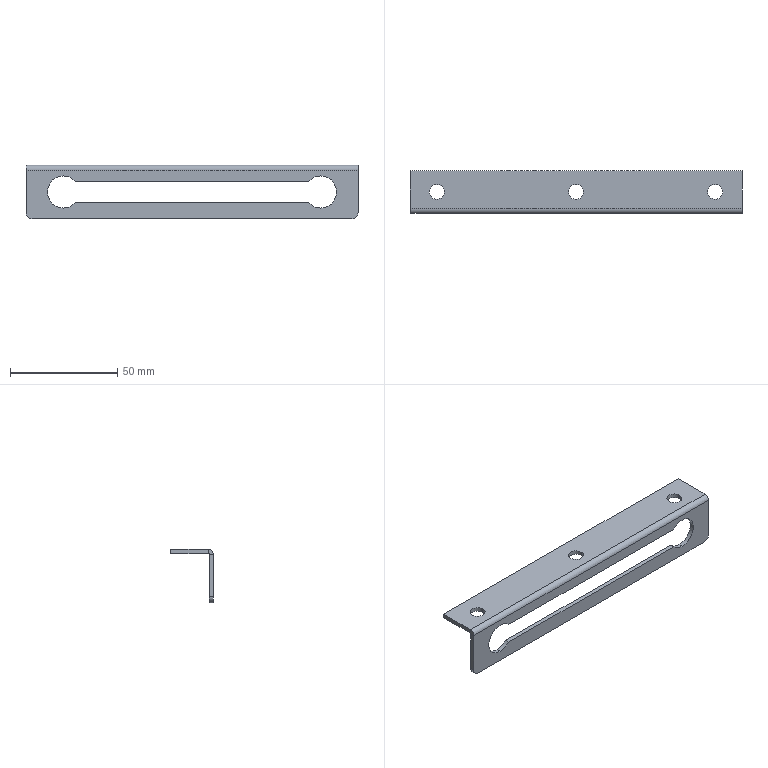Part | SolidWorks | features Cut 2, Fillet 1, FlatPattern 1, SMBaseFlange 1, SheetMetal 1 | 1 solid | 30 faces | box 155 x 20 x 25 mm | volume 10088 mm3 | cylinder 16 | plane 14 | commonest cylinder face diameters 7 x6 15 x6 6 x2 0.6 x1 4.6 x1
STEP:
#1=CARTESIAN_POINT('',(131.91,-18.,-7.5));
#2=VERTEX_POINT('',#1);
#3=CARTESIAN_POINT('',(137.5,-18.,-5.));
#4=VERTEX_POINT('',#3);
#5=CARTESIAN_POINT('',(137.5,-18.,-12.5));
#6=DIRECTION('',(0.,1.,0.));
#7=DIRECTION('',(0.,0.,1.));
#8=AXIS2_PLACEMENT_3D('',#5,#6,#7);
#9=CIRCLE('',#8,7.5);
#10=EDGE_CURVE('',#2,#4,#9,.T.);
#11=ORIENTED_EDGE('',*,*,#10,.T.);
#12=CARTESIAN_POINT('',(137.5,-20.,-5.));
#13=VERTEX_POINT('',#12);
#14=CARTESIAN_POINT('',(137.5,-10.,-5.));
#15=DIRECTION('',(0.,-1.,0.));
#16=VECTOR('',#15,1000.);
#17=LINE('',#14,#16);
#18=EDGE_CURVE('',#4,#13,#17,.T.);
#19=ORIENTED_EDGE('',*,*,#18,.T.);
#20=CARTESIAN_POINT('',(131.91,-20.,-7.5));
#21=VERTEX_POINT('',#20);
#22=CARTESIAN_POINT('',(137.5,-20.,-12.5));
#23=DIRECTION('',(0.,-1.,0.));
#24=DIRECTION('',(0.,0.,1.));
#25=AXIS2_PLACEMENT_3D('',#22,#23,#24);
#26=CIRCLE('',#25,7.5);
#27=EDGE_CURVE('',#13,#21,#26,.T.);
#28=ORIENTED_EDGE('',*,*,#27,.T.);
#29=CARTESIAN_POINT('',(131.91,-10.,-7.5));
#30=DIRECTION('',(0.,-1.,0.));
#31=VECTOR('',#30,1000.);
#32=LINE('',#29,#31);
#33=EDGE_CURVE('',#2,#21,#32,.T.);
#34=ORIENTED_EDGE('',*,*,#33,.F.);
#35=EDGE_LOOP('',(#11,#19,#28,#34));
#36=FACE_OUTER_BOUND('',#35,.T.);
#37=CARTESIAN_POINT('',(137.5,-10.,-12.5));
#38=DIRECTION('',(0.,-1.,0.));
#39=DIRECTION('',(0.,0.,-1.));
#40=AXIS2_PLACEMENT_3D('',#37,#38,#39);
#41=CYLINDRICAL_SURFACE('',#40,7.5);
#42=ADVANCED_FACE('',(#36),#41,.F.);
#43=ORIENTED_EDGE('',*,*,#18,.F.);
#44=CARTESIAN_POINT('',(137.5,-18.,-20.));
#45=VERTEX_POINT('',#44);
#46=CARTESIAN_POINT('',(137.5,-18.,-12.5));
#47=DIRECTION('',(0.,1.,0.));
#48=DIRECTION('',(0.,0.,1.));
#49=AXIS2_PLACEMENT_3D('',#46,#47,#48);
#50=CIRCLE('',#49,7.5);
#51=EDGE_CURVE('',#4,#45,#50,.T.);
#52=ORIENTED_EDGE('',*,*,#51,.T.);
#53=CARTESIAN_POINT('',(137.5,-20.,-20.));
#54=VERTEX_POINT('',#53);
#55=CARTESIAN_POINT('',(137.5,-10.,-20.));
#56=DIRECTION('',(0.,-1.,0.));
#57=VECTOR('',#56,1000.);
#58=LINE('',#55,#57);
#59=EDGE_CURVE('',#45,#54,#58,.T.);
#60=ORIENTED_EDGE('',*,*,#59,.T.);
#61=CARTESIAN_POINT('',(137.5,-20.,-12.5));
#62=DIRECTION('',(0.,-1.,0.));
#63=DIRECTION('',(0.,0.,1.));
#64=AXIS2_PLACEMENT_3D('',#61,#62,#63);
#65=CIRCLE('',#64,7.5);
#66=EDGE_CURVE('',#54,#13,#65,.T.);
#67=ORIENTED_EDGE('',*,*,#66,.T.);
#68=EDGE_LOOP('',(#43,#52,#60,#67));
#69=FACE_OUTER_BOUND('',#68,.T.);
#70=CARTESIAN_POINT('',(137.5,-10.,-12.5));
#71=DIRECTION('',(0.,-1.,0.));
#72=DIRECTION('',(0.,0.,-1.));
#73=AXIS2_PLACEMENT_3D('',#70,#71,#72);
#74=CYLINDRICAL_SURFACE('',#73,7.5);
#75=ADVANCED_FACE('',(#69),#74,.F.);
#76=CARTESIAN_POINT('',(17.5,-18.,-20.));
#77=VERTEX_POINT('',#76);
#78=CARTESIAN_POINT('',(17.5,-18.,-5.));
#79=VERTEX_POINT('',#78);
#80=CARTESIAN_POINT('',(17.5,-18.,-12.5));
#81=DIRECTION('',(0.,1.,0.));
#82=DIRECTION('',(0.,0.,1.));
#83=AXIS2_PLACEMENT_3D('',#80,#81,#82);
#84=CIRCLE('',#83,7.5);
#85=EDGE_CURVE('',#77,#79,#84,.T.);
#86=ORIENTED_EDGE('',*,*,#85,.T.);
#87=CARTESIAN_POINT('',(17.5,-20.,-5.));
#88=VERTEX_POINT('',#87);
#89=CARTESIAN_POINT('',(17.5,-10.,-5.));
#90=DIRECTION('',(0.,-1.,0.));
#91=VECTOR('',#90,1000.);
#92=LINE('',#89,#91);
#93=EDGE_CURVE('',#79,#88,#92,.T.);
#94=ORIENTED_EDGE('',*,*,#93,.T.);
#95=CARTESIAN_POINT('',(17.5,-20.,-20.));
#96=VERTEX_POINT('',#95);
#97=CARTESIAN_POINT('',(17.5,-20.,-12.5));
#98=DIRECTION('',(0.,-1.,0.));
#99=DIRECTION('',(0.,0.,-1.));
#100=AXIS2_PLACEMENT_3D('',#97,#98,#99);
#101=CIRCLE('',#100,7.5);
#102=EDGE_CURVE('',#88,#96,#101,.T.);
#103=ORIENTED_EDGE('',*,*,#102,.T.);
#104=CARTESIAN_POINT('',(17.5,-10.,-20.));
#105=DIRECTION('',(0.,-1.,0.));
#106=VECTOR('',#105,1000.);
#107=LINE('',#104,#106);
#108=EDGE_CURVE('',#77,#96,#107,.T.);
#109=ORIENTED_EDGE('',*,*,#108,.F.);
#110=EDGE_LOOP('',(#86,#94,#103,#109));
#111=FACE_OUTER_BOUND('',#110,.T.);
#112=CARTESIAN_POINT('',(17.5,-10.,-12.5));
#113=DIRECTION('',(0.,-1.,0.));
#114=DIRECTION('',(0.,0.,-1.));
#115=AXIS2_PLACEMENT_3D('',#112,#113,#114);
#116=CYLINDRICAL_SURFACE('',#115,7.5);
#117=ADVANCED_FACE('',(#111),#116,.F.);
#118=CARTESIAN_POINT('',(23.09,-18.,-17.5));
#119=VERTEX_POINT('',#118);
#120=CARTESIAN_POINT('',(17.5,-18.,-12.5));
#121=DIRECTION('',(0.,1.,0.));
#122=DIRECTION('',(0.,0.,1.));
#123=AXIS2_PLACEMENT_3D('',#120,#121,#122);
#124=CIRCLE('',#123,7.5);
#125=EDGE_CURVE('',#119,#77,#124,.T.);
#126=ORIENTED_EDGE('',*,*,#125,.T.);
#127=ORIENTED_EDGE('',*,*,#108,.T.);
#128=CARTESIAN_POINT('',(23.09,-20.,-17.5));
#129=VERTEX_POINT('',#128);
#130=CARTESIAN_POINT('',(17.5,-20.,-12.5));
#131=DIRECTION('',(0.,-1.,0.));
#132=DIRECTION('',(0.,0.,-1.));
#133=AXIS2_PLACEMENT_3D('',#130,#131,#132);
#134=CIRCLE('',#133,7.5);
#135=EDGE_CURVE('',#96,#129,#134,.T.);
#136=ORIENTED_EDGE('',*,*,#135,.T.);
#137=CARTESIAN_POINT('',(23.09,-10.,-17.5));
#138=DIRECTION('',(0.,-1.,0.));
#139=VECTOR('',#138,1000.);
#140=LINE('',#137,#139);
#141=EDGE_CURVE('',#119,#129,#140,.T.);
#142=ORIENTED_EDGE('',*,*,#141,.F.);
#143=EDGE_LOOP('',(#126,#127,#136,#142));
#144=FACE_OUTER_BOUND('',#143,.T.);
#145=CARTESIAN_POINT('',(17.5,-10.,-12.5));
#146=DIRECTION('',(0.,-1.,0.));
#147=DIRECTION('',(0.,0.,-1.));
#148=AXIS2_PLACEMENT_3D('',#145,#146,#147);
#149=CYLINDRICAL_SURFACE('',#148,7.5);
#150=ADVANCED_FACE('',(#144),#149,.F.);
#151=CARTESIAN_POINT('',(146.,-10.,-2.));
#152=VERTEX_POINT('',#151);
#153=CARTESIAN_POINT('',(139.,-10.,-2.));
#154=VERTEX_POINT('',#153);
#155=CARTESIAN_POINT('',(142.5,-10.,-2.));
#156=DIRECTION('',(0.,0.,-1.));
#157=DIRECTION('',(0.,1.,0.));
#158=AXIS2_PLACEMENT_3D('',#155,#156,#157);
#159=CIRCLE('',#158,3.5);
#160=EDGE_CURVE('',#152,#154,#159,.T.);
#161=ORIENTED_EDGE('',*,*,#160,.T.);
#162=CARTESIAN_POINT('',(139.,-10.,0.));
#163=VERTEX_POINT('',#162);
#164=CARTESIAN_POINT('',(139.,-10.,-10.));
#165=DIRECTION('',(0.,0.,1.));
#166=VECTOR('',#165,1000.);
#167=LINE('',#164,#166);
#168=EDGE_CURVE('',#154,#163,#167,.T.);
#169=ORIENTED_EDGE('',*,*,#168,.T.);
#170=CARTESIAN_POINT('',(146.,-10.,0.));
#171=VERTEX_POINT('',#170);
#172=CARTESIAN_POINT('',(142.5,-10.,0.));
#173=DIRECTION('',(0.,0.,1.));
#174=DIRECTION('',(1.,0.,0.));
#175=AXIS2_PLACEMENT_3D('',#172,#173,#174);
#176=CIRCLE('',#175,3.5);
#177=EDGE_CURVE('',#163,#171,#176,.T.);
#178=ORIENTED_EDGE('',*,*,#177,.T.);
#179=CARTESIAN_POINT('',(146.,-10.,-10.));
#180=DIRECTION('',(0.,0.,1.));
#181=VECTOR('',#180,1000.);
#182=LINE('',#179,#181);
#183=EDGE_CURVE('',#152,#171,#182,.T.);
#184=ORIENTED_EDGE('',*,*,#183,.F.);
#185=EDGE_LOOP('',(#161,#169,#178,#184));
#186=FACE_OUTER_BOUND('',#185,.T.);
#187=CARTESIAN_POINT('',(142.5,-10.,-10.));
#188=DIRECTION('',(0.,0.,1.));
#189=DIRECTION('',(1.,0.,0.));
#190=AXIS2_PLACEMENT_3D('',#187,#188,#189);
#191=CYLINDRICAL_SURFACE('',#190,3.5);
#192=ADVANCED_FACE('',(#186),#191,.F.);
#193=CARTESIAN_POINT('',(81.,-10.,-2.));
#194=VERTEX_POINT('',#193);
#195=CARTESIAN_POINT('',(74.,-10.,-2.));
#196=VERTEX_POINT('',#195);
#197=CARTESIAN_POINT('',(77.5,-10.,-2.));
#198=DIRECTION('',(0.,0.,-1.));
#199=DIRECTION('',(0.,1.,0.));
#200=AXIS2_PLACEMENT_3D('',#197,#198,#199);
#201=CIRCLE('',#200,3.5);
#202=EDGE_CURVE('',#194,#196,#201,.T.);
#203=ORIENTED_EDGE('',*,*,#202,.T.);
#204=CARTESIAN_POINT('',(74.,-10.,0.));
#205=VERTEX_POINT('',#204);
#206=CARTESIAN_POINT('',(74.,-10.,-10.));
#207=DIRECTION('',(0.,0.,1.));
#208=VECTOR('',#207,1000.);
#209=LINE('',#206,#208);
#210=EDGE_CURVE('',#196,#205,#209,.T.);
#211=ORIENTED_EDGE('',*,*,#210,.T.);
#212=CARTESIAN_POINT('',(81.,-10.,0.));
#213=VERTEX_POINT('',#212);
#214=CARTESIAN_POINT('',(77.5,-10.,0.));
#215=DIRECTION('',(0.,0.,1.));
#216=DIRECTION('',(1.,0.,0.));
#217=AXIS2_PLACEMENT_3D('',#214,#215,#216);
#218=CIRCLE('',#217,3.5);
#219=EDGE_CURVE('',#205,#213,#218,.T.);
#220=ORIENTED_EDGE('',*,*,#219,.T.);
#221=CARTESIAN_POINT('',(81.,-10.,-10.));
#222=DIRECTION('',(0.,0.,1.));
#223=VECTOR('',#222,1000.);
#224=LINE('',#221,#223);
#225=EDGE_CURVE('',#194,#213,#224,.T.);
#226=ORIENTED_EDGE('',*,*,#225,.F.);
#227=EDGE_LOOP('',(#203,#211,#220,#226));
#228=FACE_OUTER_BOUND('',#227,.T.);
#229=CARTESIAN_POINT('',(77.5,-10.,-10.));
#230=DIRECTION('',(0.,0.,1.));
#231=DIRECTION('',(1.,0.,0.));
#232=AXIS2_PLACEMENT_3D('',#229,#230,#231);
#233=CYLINDRICAL_SURFACE('',#232,3.5);
#234=ADVANCED_FACE('',(#228),#233,.F.);
#235=CARTESIAN_POINT('',(16.,-10.,-2.));
#236=VERTEX_POINT('',#235);
#237=CARTESIAN_POINT('',(9.,-10.,-2.));
#238=VERTEX_POINT('',#237);
#239=CARTESIAN_POINT('',(12.5,-10.,-2.));
#240=DIRECTION('',(0.,0.,-1.));
#241=DIRECTION('',(0.,1.,0.));
#242=AXIS2_PLACEMENT_3D('',#239,#240,#241);
#243=CIRCLE('',#242,3.5);
#244=EDGE_CURVE('',#236,#238,#243,.T.);
#245=ORIENTED_EDGE('',*,*,#244,.T.);
#246=CARTESIAN_POINT('',(9.,-10.,0.));
#247=VERTEX_POINT('',#246);
#248=CARTESIAN_POINT('',(9.,-10.,-10.));
#249=DIRECTION('',(0.,0.,1.));
#250=VECTOR('',#249,1000.);
#251=LINE('',#248,#250);
#252=EDGE_CURVE('',#238,#247,#251,.T.);
#253=ORIENTED_EDGE('',*,*,#252,.T.);
#254=CARTESIAN_POINT('',(16.,-10.,0.));
#255=VERTEX_POINT('',#254);
#256=CARTESIAN_POINT('',(12.5,-10.,0.));
#257=DIRECTION('',(0.,0.,1.));
#258=DIRECTION('',(1.,0.,0.));
#259=AXIS2_PLACEMENT_3D('',#256,#257,#258);
#260=CIRCLE('',#259,3.5);
#261=EDGE_CURVE('',#247,#255,#260,.T.);
#262=ORIENTED_EDGE('',*,*,#261,.T.);
#263=CARTESIAN_POINT('',(16.,-10.,-10.));
#264=DIRECTION('',(0.,0.,1.));
#265=VECTOR('',#264,1000.);
#266=LINE('',#263,#265);
#267=EDGE_CURVE('',#236,#255,#266,.T.);
#268=ORIENTED_EDGE('',*,*,#267,.F.);
#269=EDGE_LOOP('',(#245,#253,#262,#268));
#270=FACE_OUTER_BOUND('',#269,.T.);
#271=CARTESIAN_POINT('',(12.5,-10.,-10.));
#272=DIRECTION('',(0.,0.,1.));
#273=DIRECTION('',(1.,0.,0.));
#274=AXIS2_PLACEMENT_3D('',#271,#272,#273);
#275=CYLINDRICAL_SURFACE('',#274,3.5);
#276=ADVANCED_FACE('',(#270),#275,.F.);
#277=CARTESIAN_POINT('',(155.,-17.7,0.));
#278=VERTEX_POINT('',#277);
#279=CARTESIAN_POINT('',(155.,-17.7,-2.));
#280=VERTEX_POINT('',#279);
#281=CARTESIAN_POINT('',(155.,-17.7,0.));
#282=DIRECTION('',(0.,0.,-1.));
#283=VECTOR('',#282,1000.);
#284=LINE('',#281,#283);
#285=EDGE_CURVE('',#278,#280,#284,.T.);
#286=ORIENTED_EDGE('',*,*,#285,.F.);
#287=CARTESIAN_POINT('',(155.,-20.,-2.3));
#288=VERTEX_POINT('',#287);
#289=CARTESIAN_POINT('',(155.,-17.7,-2.3));
#290=DIRECTION('',(1.,0.,0.));
#291=DIRECTION('',(0.,0.,1.));
#292=AXIS2_PLACEMENT_3D('',#289,#290,#291);
#293=CIRCLE('',#292,2.3);
#294=EDGE_CURVE('',#278,#288,#293,.T.);
#295=ORIENTED_EDGE('',*,*,#294,.T.);
#296=CARTESIAN_POINT('',(155.,-18.,-2.3));
#297=VERTEX_POINT('',#296);
#298=CARTESIAN_POINT('',(155.,-18.,-2.3));
#299=DIRECTION('',(0.,-1.,0.));
#300=VECTOR('',#299,1000.);
#301=LINE('',#298,#300);
#302=EDGE_CURVE('',#297,#288,#301,.T.);
#303=ORIENTED_EDGE('',*,*,#302,.F.);
#304=CARTESIAN_POINT('',(155.,-17.7,-2.3));
#305=DIRECTION('',(1.,0.,0.));
#306=DIRECTION('',(0.,0.,-1.));
#307=AXIS2_PLACEMENT_3D('',#304,#305,#306);
#308=CIRCLE('',#307,0.3);
#309=EDGE_CURVE('',#280,#297,#308,.T.);
#310=ORIENTED_EDGE('',*,*,#309,.F.);
#311=EDGE_LOOP('',(#286,#295,#303,#310));
#312=FACE_OUTER_BOUND('',#311,.T.);
#313=CARTESIAN_POINT('',(155.,-17.7,0.));
#314=DIRECTION('',(1.,0.,0.));
#315=DIRECTION('',(0.,0.,-1.));
#316=AXIS2_PLACEMENT_3D('',#313,#314,#315);
#317=PLANE('',#316);
#318=ADVANCED_FACE('',(#312),#317,.T.);
#319=CARTESIAN_POINT('',(155.,0.,0.));
#320=VERTEX_POINT('',#319);
#321=CARTESIAN_POINT('',(155.,0.,0.));
#322=DIRECTION('',(0.,-1.,0.));
#323=VECTOR('',#322,1000.);
#324=LINE('',#321,#323);
#325=EDGE_CURVE('',#320,#278,#324,.T.);
#326=ORIENTED_EDGE('',*,*,#325,.T.);
#327=ORIENTED_EDGE('',*,*,#285,.T.);
#328=CARTESIAN_POINT('',(155.,0.,-2.));
#329=VERTEX_POINT('',#328);
#330=CARTESIAN_POINT('',(155.,0.,-2.));
#331=DIRECTION('',(0.,-1.,0.));
#332=VECTOR('',#331,1000.);
#333=LINE('',#330,#332);
#334=EDGE_CURVE('',#329,#280,#333,.T.);
#335=ORIENTED_EDGE('',*,*,#334,.F.);
#336=CARTESIAN_POINT('',(155.,0.,0.));
#337=DIRECTION('',(0.,0.,-1.));
#338=VECTOR('',#337,1000.);
#339=LINE('',#336,#338);
#340=EDGE_CURVE('',#320,#329,#339,.T.);
#341=ORIENTED_EDGE('',*,*,#340,.F.);
#342=EDGE_LOOP('',(#326,#327,#335,#341));
#343=FACE_OUTER_BOUND('',#342,.T.);
#344=CARTESIAN_POINT('',(155.,-18.,-2.3));
#345=DIRECTION('',(1.,0.,0.));
#346=DIRECTION('',(0.,0.,-1.));
#347=AXIS2_PLACEMENT_3D('',#344,#345,#346);
#348=PLANE('',#347);
#349=ADVANCED_FACE('',(#343),#348,.T.);
#350=CARTESIAN_POINT('',(0.,-20.,-2.3));
#351=VERTEX_POINT('',#350);
#352=CARTESIAN_POINT('',(0.,-18.,-2.3));
#353=VERTEX_POINT('',#352);
#354=CARTESIAN_POINT('',(0.,-20.,-2.3));
#355=DIRECTION('',(0.,1.,0.));
#356=VECTOR('',#355,1000.);
#357=LINE('',#354,#356);
#358=EDGE_CURVE('',#351,#353,#357,.T.);
#359=ORIENTED_EDGE('',*,*,#358,.F.);
#360=CARTESIAN_POINT('',(0.,-17.7,0.));
#361=VERTEX_POINT('',#360);
#362=CARTESIAN_POINT('',(0.,-17.7,-2.3));
#363=DIRECTION('',(1.,0.,0.));
#364=DIRECTION('',(0.,0.,1.));
#365=AXIS2_PLACEMENT_3D('',#362,#363,#364);
#366=CIRCLE('',#365,2.3);
#367=EDGE_CURVE('',#361,#351,#366,.T.);
#368=ORIENTED_EDGE('',*,*,#367,.F.);
#369=CARTESIAN_POINT('',(0.,-17.7,-2.));
#370=VERTEX_POINT('',#369);
#371=CARTESIAN_POINT('',(0.,-17.7,-2.));
#372=DIRECTION('',(0.,0.,1.));
#373=VECTOR('',#372,1000.);
#374=LINE('',#371,#373);
#375=EDGE_CURVE('',#370,#361,#374,.T.);
#376=ORIENTED_EDGE('',*,*,#375,.F.);
#377=CARTESIAN_POINT('',(0.,-17.7,-2.3));
#378=DIRECTION('',(1.,0.,0.));
#379=DIRECTION('',(0.,0.,-1.));
#380=AXIS2_PLACEMENT_3D('',#377,#378,#379);
#381=CIRCLE('',#380,0.3);
#382=EDGE_CURVE('',#370,#353,#381,.T.);
#383=ORIENTED_EDGE('',*,*,#382,.T.);
#384=EDGE_LOOP('',(#359,#368,#376,#383));
#385=FACE_OUTER_BOUND('',#384,.T.);
#386=CARTESIAN_POINT('',(0.,-20.,-2.3));
#387=DIRECTION('',(-1.,0.,0.));
#388=DIRECTION('',(0.,0.,1.));
#389=AXIS2_PLACEMENT_3D('',#386,#387,#388);
#390=PLANE('',#389);
#391=ADVANCED_FACE('',(#385),#390,.T.);
#392=CARTESIAN_POINT('',(0.,-18.,-22.));
#393=VERTEX_POINT('',#392);
#394=CARTESIAN_POINT('',(0.,-18.,0.));
#395=DIRECTION('',(0.,0.,-1.));
#396=VECTOR('',#395,1000.);
#397=LINE('',#394,#396);
#398=EDGE_CURVE('',#353,#393,#397,.T.);
#399=ORIENTED_EDGE('',*,*,#398,.T.);
#400=CARTESIAN_POINT('',(0.,-20.,-22.));
#401=VERTEX_POINT('',#400);
#402=CARTESIAN_POINT('',(0.,-17.7,-22.));
#403=DIRECTION('',(0.,-1.,0.));
#404=VECTOR('',#403,1000.);
#405=LINE('',#402,#404);
#406=EDGE_CURVE('',#393,#401,#405,.T.);
#407=ORIENTED_EDGE('',*,*,#406,.T.);
#408=CARTESIAN_POINT('',(0.,-20.,0.));
#409=DIRECTION('',(0.,0.,-1.));
#410=VECTOR('',#409,1000.);
#411=LINE('',#408,#410);
#412=EDGE_CURVE('',#351,#401,#411,.T.);
#413=ORIENTED_EDGE('',*,*,#412,.F.);
#414=ORIENTED_EDGE('',*,*,#358,.T.);
#415=EDGE_LOOP('',(#399,#407,#413,#414));
#416=FACE_OUTER_BOUND('',#415,.T.);
#417=CARTESIAN_POINT('',(0.,-17.7,-2.));
#418=DIRECTION('',(-1.,0.,0.));
#419=DIRECTION('',(0.,0.,1.));
#420=AXIS2_PLACEMENT_3D('',#417,#418,#419);
#421=PLANE('',#420);
#422=ADVANCED_FACE('',(#416),#421,.T.);
#423=CARTESIAN_POINT('',(131.91,-20.,-17.5));
#424=VERTEX_POINT('',#423);
#425=CARTESIAN_POINT('',(23.09,-20.,-17.5));
#426=DIRECTION('',(1.,0.,0.));
#427=VECTOR('',#426,1000.);
#428=LINE('',#425,#427);
#429=EDGE_CURVE('',#129,#424,#428,.T.);
#430=ORIENTED_EDGE('',*,*,#429,.F.);
#431=ORIENTED_EDGE('',*,*,#135,.F.);
#432=ORIENTED_EDGE('',*,*,#102,.F.);
#433=CARTESIAN_POINT('',(23.09,-20.,-7.5));
#434=VERTEX_POINT('',#433);
#435=CARTESIAN_POINT('',(17.5,-20.,-12.5));
#436=DIRECTION('',(0.,-1.,0.));
#437=DIRECTION('',(0.,0.,-1.));
#438=AXIS2_PLACEMENT_3D('',#435,#436,#437);
#439=CIRCLE('',#438,7.5);
#440=EDGE_CURVE('',#434,#88,#439,.T.);
#441=ORIENTED_EDGE('',*,*,#440,.F.);
#442=CARTESIAN_POINT('',(23.09,-20.,-7.5));
#443=DIRECTION('',(-1.,0.,0.));
#444=VECTOR('',#443,1000.);
#445=LINE('',#442,#444);
#446=EDGE_CURVE('',#21,#434,#445,.T.);
#447=ORIENTED_EDGE('',*,*,#446,.F.);
#448=ORIENTED_EDGE('',*,*,#27,.F.);
#449=ORIENTED_EDGE('',*,*,#66,.F.);
#450=CARTESIAN_POINT('',(137.5,-20.,-12.5));
#451=DIRECTION('',(0.,-1.,0.));
#452=DIRECTION('',(0.,0.,1.));
#453=AXIS2_PLACEMENT_3D('',#450,#451,#452);
#454=CIRCLE('',#453,7.5);
#455=EDGE_CURVE('',#424,#54,#454,.T.);
#456=ORIENTED_EDGE('',*,*,#455,.F.);
#457=EDGE_LOOP('',(#430,#431,#432,#441,#447,#448,#449,#456));
#458=FACE_BOUND('',#457,.T.);
#459=ORIENTED_EDGE('',*,*,#412,.T.);
#460=CARTESIAN_POINT('',(3.,-20.,-25.));
#461=VERTEX_POINT('',#460);
#462=CARTESIAN_POINT('',(3.,-20.,-22.));
#463=DIRECTION('',(0.,-1.,0.));
#464=DIRECTION('',(0.,0.,1.));
#465=AXIS2_PLACEMENT_3D('',#462,#463,#464);
#466=CIRCLE('',#465,3.);
#467=EDGE_CURVE('',#401,#461,#466,.T.);
#468=ORIENTED_EDGE('',*,*,#467,.T.);
#469=CARTESIAN_POINT('',(152.,-20.,-25.));
#470=VERTEX_POINT('',#469);
#471=CARTESIAN_POINT('',(155.,-20.,-25.));
#472=DIRECTION('',(-1.,0.,0.));
#473=VECTOR('',#472,1000.);
#474=LINE('',#471,#473);
#475=EDGE_CURVE('',#470,#461,#474,.T.);
#476=ORIENTED_EDGE('',*,*,#475,.F.);
#477=CARTESIAN_POINT('',(155.,-20.,-22.));
#478=VERTEX_POINT('',#477);
#479=CARTESIAN_POINT('',(152.,-20.,-22.));
#480=DIRECTION('',(0.,-1.,0.));
#481=DIRECTION('',(0.,0.,1.));
#482=AXIS2_PLACEMENT_3D('',#479,#480,#481);
#483=CIRCLE('',#482,3.);
#484=EDGE_CURVE('',#470,#478,#483,.T.);
#485=ORIENTED_EDGE('',*,*,#484,.T.);
#486=CARTESIAN_POINT('',(155.,-20.,0.));
#487=DIRECTION('',(0.,0.,-1.));
#488=VECTOR('',#487,1000.);
#489=LINE('',#486,#488);
#490=EDGE_CURVE('',#288,#478,#489,.T.);
#491=ORIENTED_EDGE('',*,*,#490,.F.);
#492=CARTESIAN_POINT('',(155.,-20.,-2.3));
#493=DIRECTION('',(-1.,0.,0.));
#494=VECTOR('',#493,1000.);
#495=LINE('',#492,#494);
#496=EDGE_CURVE('',#288,#351,#495,.T.);
#497=ORIENTED_EDGE('',*,*,#496,.T.);
#498=EDGE_LOOP('',(#459,#468,#476,#485,#491,#497));
#499=FACE_OUTER_BOUND('',#498,.T.);
#500=CARTESIAN_POINT('',(155.,-20.,0.));
#501=DIRECTION('',(0.,1.,0.));
#502=DIRECTION('',(0.,0.,1.));
#503=AXIS2_PLACEMENT_3D('',#500,#501,#502);
#504=PLANE('',#503);
#505=ADVANCED_FACE('',(#458,#499),#504,.F.);
#506=ORIENTED_EDGE('',*,*,#475,.T.);
#507=CARTESIAN_POINT('',(3.,-18.,-25.));
#508=VERTEX_POINT('',#507);
#509=CARTESIAN_POINT('',(3.,-18.,-25.));
#510=DIRECTION('',(0.,1.,0.));
#511=VECTOR('',#510,1000.);
#512=LINE('',#509,#511);
#513=EDGE_CURVE('',#461,#508,#512,.T.);
#514=ORIENTED_EDGE('',*,*,#513,.T.);
#515=CARTESIAN_POINT('',(152.,-18.,-25.));
#516=VERTEX_POINT('',#515);
#517=CARTESIAN_POINT('',(155.,-18.,-25.));
#518=DIRECTION('',(-1.,0.,0.));
#519=VECTOR('',#518,1000.);
#520=LINE('',#517,#519);
#521=EDGE_CURVE('',#516,#508,#520,.T.);
#522=ORIENTED_EDGE('',*,*,#521,.F.);
#523=CARTESIAN_POINT('',(152.,-18.,-25.));
#524=DIRECTION('',(0.,-1.,0.));
#525=VECTOR('',#524,1000.);
#526=LINE('',#523,#525);
#527=EDGE_CURVE('',#516,#470,#526,.T.);
#528=ORIENTED_EDGE('',*,*,#527,.T.);
#529=EDGE_LOOP('',(#506,#514,#522,#528));
#530=FACE_OUTER_BOUND('',#529,.T.);
#531=CARTESIAN_POINT('',(155.,-18.,-25.));
#532=DIRECTION('',(0.,0.,-1.));
#533=DIRECTION('',(-1.,0.,0.));
#534=AXIS2_PLACEMENT_3D('',#531,#532,#533);
#535=PLANE('',#534);
#536=ADVANCED_FACE('',(#530),#535,.T.);
#537=ORIENTED_EDGE('',*,*,#125,.F.);
#538=CARTESIAN_POINT('',(131.91,-18.,-17.5));
#539=VERTEX_POINT('',#538);
#540=CARTESIAN_POINT('',(155.,-18.,-17.5));
#541=DIRECTION('',(-1.,0.,0.));
#542=VECTOR('',#541,1000.);
#543=LINE('',#540,#542);
#544=EDGE_CURVE('',#539,#119,#543,.T.);
#545=ORIENTED_EDGE('',*,*,#544,.F.);
#546=CARTESIAN_POINT('',(137.5,-18.,-12.5));
#547=DIRECTION('',(0.,1.,0.));
#548=DIRECTION('',(0.,0.,1.));
#549=AXIS2_PLACEMENT_3D('',#546,#547,#548);
#550=CIRCLE('',#549,7.5);
#551=EDGE_CURVE('',#45,#539,#550,.T.);
#552=ORIENTED_EDGE('',*,*,#551,.F.);
#553=ORIENTED_EDGE('',*,*,#51,.F.);
#554=ORIENTED_EDGE('',*,*,#10,.F.);
#555=CARTESIAN_POINT('',(23.09,-18.,-7.5));
#556=VERTEX_POINT('',#555);
#557=CARTESIAN_POINT('',(155.,-18.,-7.5));
#558=DIRECTION('',(1.,0.,0.));
#559=VECTOR('',#558,1000.);
#560=LINE('',#557,#559);
#561=EDGE_CURVE('',#556,#2,#560,.T.);
#562=ORIENTED_EDGE('',*,*,#561,.F.);
#563=CARTESIAN_POINT('',(17.5,-18.,-12.5));
#564=DIRECTION('',(0.,1.,0.));
#565=DIRECTION('',(0.,0.,1.));
#566=AXIS2_PLACEMENT_3D('',#563,#564,#565);
#567=CIRCLE('',#566,7.5);
#568=EDGE_CURVE('',#79,#556,#567,.T.);
#569=ORIENTED_EDGE('',*,*,#568,.F.);
#570=ORIENTED_EDGE('',*,*,#85,.F.);
#571=EDGE_LOOP('',(#537,#545,#552,#553,#554,#562,#569,#570));
#572=FACE_BOUND('',#571,.T.);
#573=ORIENTED_EDGE('',*,*,#521,.T.);
#574=CARTESIAN_POINT('',(3.,-18.,-22.));
#575=DIRECTION('',(0.,1.,0.));
#576=DIRECTION('',(0.,0.,1.));
#577=AXIS2_PLACEMENT_3D('',#574,#575,#576);
#578=CIRCLE('',#577,3.);
#579=EDGE_CURVE('',#508,#393,#578,.T.);
#580=ORIENTED_EDGE('',*,*,#579,.T.);
#581=ORIENTED_EDGE('',*,*,#398,.F.);
#582=CARTESIAN_POINT('',(155.,-18.,-2.3));
#583=DIRECTION('',(-1.,0.,0.));
#584=VECTOR('',#583,1000.);
#585=LINE('',#582,#584);
#586=EDGE_CURVE('',#297,#353,#585,.T.);
#587=ORIENTED_EDGE('',*,*,#586,.F.);
#588=CARTESIAN_POINT('',(155.,-18.,-22.));
#589=VERTEX_POINT('',#588);
#590=CARTESIAN_POINT('',(155.,-18.,0.));
#591=DIRECTION('',(0.,0.,-1.));
#592=VECTOR('',#591,1000.);
#593=LINE('',#590,#592);
#594=EDGE_CURVE('',#297,#589,#593,.T.);
#595=ORIENTED_EDGE('',*,*,#594,.T.);
#596=CARTESIAN_POINT('',(152.,-18.,-22.));
#597=DIRECTION('',(0.,1.,0.));
#598=DIRECTION('',(0.,0.,1.));
#599=AXIS2_PLACEMENT_3D('',#596,#597,#598);
#600=CIRCLE('',#599,3.);
#601=EDGE_CURVE('',#589,#516,#600,.T.);
#602=ORIENTED_EDGE('',*,*,#601,.T.);
#603=EDGE_LOOP('',(#573,#580,#581,#587,#595,#602));
#604=FACE_OUTER_BOUND('',#603,.T.);
#605=CARTESIAN_POINT('',(155.,-18.,0.));
#606=DIRECTION('',(0.,1.,0.));
#607=DIRECTION('',(0.,0.,1.));
#608=AXIS2_PLACEMENT_3D('',#605,#606,#607);
#609=PLANE('',#608);
#610=ADVANCED_FACE('',(#572,#604),#609,.T.);
#611=ORIENTED_EDGE('',*,*,#382,.F.);
#612=CARTESIAN_POINT('',(155.,-17.7,-2.));
#613=DIRECTION('',(-1.,0.,0.));
#614=VECTOR('',#613,1000.);
#615=LINE('',#612,#614);
#616=EDGE_CURVE('',#280,#370,#615,.T.);
#617=ORIENTED_EDGE('',*,*,#616,.F.);
#618=ORIENTED_EDGE('',*,*,#309,.T.);
#619=ORIENTED_EDGE('',*,*,#586,.T.);
#620=EDGE_LOOP('',(#611,#617,#618,#619));
#621=FACE_OUTER_BOUND('',#620,.T.);
#622=CARTESIAN_POINT('',(155.,-17.7,-2.3));
#623=DIRECTION('',(-1.,0.,0.));
#624=DIRECTION('',(0.,0.,1.));
#625=AXIS2_PLACEMENT_3D('',#622,#623,#624);
#626=CYLINDRICAL_SURFACE('',#625,0.3);
#627=ADVANCED_FACE('',(#621),#626,.F.);
#628=ORIENTED_EDGE('',*,*,#160,.F.);
#629=CARTESIAN_POINT('',(142.5,-10.,-2.));
#630=DIRECTION('',(0.,0.,-1.));
#631=DIRECTION('',(0.,1.,0.));
#632=AXIS2_PLACEMENT_3D('',#629,#630,#631);
#633=CIRCLE('',#632,3.5);
#634=EDGE_CURVE('',#154,#152,#633,.T.);
#635=ORIENTED_EDGE('',*,*,#634,.F.);
#636=EDGE_LOOP('',(#628,#635));
#637=FACE_BOUND('',#636,.T.);
#638=ORIENTED_EDGE('',*,*,#202,.F.);
#639=CARTESIAN_POINT('',(77.5,-10.,-2.));
#640=DIRECTION('',(0.,0.,-1.));
#641=DIRECTION('',(0.,1.,0.));
#642=AXIS2_PLACEMENT_3D('',#639,#640,#641);
#643=CIRCLE('',#642,3.5);
#644=EDGE_CURVE('',#196,#194,#643,.T.);
#645=ORIENTED_EDGE('',*,*,#644,.F.);
#646=EDGE_LOOP('',(#638,#645));
#647=FACE_BOUND('',#646,.T.);
#648=ORIENTED_EDGE('',*,*,#244,.F.);
#649=CARTESIAN_POINT('',(12.5,-10.,-2.));
#650=DIRECTION('',(0.,0.,-1.));
#651=DIRECTION('',(0.,1.,0.));
#652=AXIS2_PLACEMENT_3D('',#649,#650,#651);
#653=CIRCLE('',#652,3.5);
#654=EDGE_CURVE('',#238,#236,#653,.T.);
#655=ORIENTED_EDGE('',*,*,#654,.F.);
#656=EDGE_LOOP('',(#648,#655));
#657=FACE_BOUND('',#656,.T.);
#658=CARTESIAN_POINT('',(0.,0.,-2.));
#659=VERTEX_POINT('',#658);
#660=CARTESIAN_POINT('',(0.,0.,-2.));
#661=DIRECTION('',(0.,-1.,0.));
#662=VECTOR('',#661,1000.);
#663=LINE('',#660,#662);
#664=EDGE_CURVE('',#659,#370,#663,.T.);
#665=ORIENTED_EDGE('',*,*,#664,.F.);
#666=CARTESIAN_POINT('',(155.,0.,-2.));
#667=DIRECTION('',(-1.,0.,0.));
#668=VECTOR('',#667,1000.);
#669=LINE('',#666,#668);
#670=EDGE_CURVE('',#329,#659,#669,.T.);
#671=ORIENTED_EDGE('',*,*,#670,.F.);
#672=ORIENTED_EDGE('',*,*,#334,.T.);
#673=ORIENTED_EDGE('',*,*,#616,.T.);
#674=EDGE_LOOP('',(#665,#671,#672,#673));
#675=FACE_OUTER_BOUND('',#674,.T.);
#676=CARTESIAN_POINT('',(155.,0.,-2.));
#677=DIRECTION('',(0.,0.,-1.));
#678=DIRECTION('',(0.,1.,0.));
#679=AXIS2_PLACEMENT_3D('',#676,#677,#678);
#680=PLANE('',#679);
#681=ADVANCED_FACE('',(#637,#647,#657,#675),#680,.T.);
#682=CARTESIAN_POINT('',(0.,0.,0.));
#683=VERTEX_POINT('',#682);
#684=CARTESIAN_POINT('',(0.,0.,0.));
#685=DIRECTION('',(0.,0.,-1.));
#686=VECTOR('',#685,1000.);
#687=LINE('',#684,#686);
#688=EDGE_CURVE('',#683,#659,#687,.T.);
#689=ORIENTED_EDGE('',*,*,#688,.F.);
#690=CARTESIAN_POINT('',(155.,0.,0.));
#691=DIRECTION('',(-1.,0.,0.));
#692=VECTOR('',#691,1000.);
#693=LINE('',#690,#692);
#694=EDGE_CURVE('',#320,#683,#693,.T.);
#695=ORIENTED_EDGE('',*,*,#694,.F.);
#696=ORIENTED_EDGE('',*,*,#340,.T.);
#697=ORIENTED_EDGE('',*,*,#670,.T.);
#698=EDGE_LOOP('',(#689,#695,#696,#697));
#699=FACE_OUTER_BOUND('',#698,.T.);
#700=CARTESIAN_POINT('',(155.,0.,0.));
#701=DIRECTION('',(0.,1.,0.));
#702=DIRECTION('',(0.,0.,1.));
#703=AXIS2_PLACEMENT_3D('',#700,#701,#702);
#704=PLANE('',#703);
#705=ADVANCED_FACE('',(#699),#704,.T.);
#706=CARTESIAN_POINT('',(142.5,-10.,0.));
#707=DIRECTION('',(0.,0.,1.));
#708=DIRECTION('',(1.,0.,0.));
#709=AXIS2_PLACEMENT_3D('',#706,#707,#708);
#710=CIRCLE('',#709,3.5);
#711=EDGE_CURVE('',#171,#163,#710,.T.);
#712=ORIENTED_EDGE('',*,*,#711,.F.);
#713=ORIENTED_EDGE('',*,*,#177,.F.);
#714=EDGE_LOOP('',(#712,#713));
#715=FACE_BOUND('',#714,.T.);
#716=CARTESIAN_POINT('',(77.5,-10.,0.));
#717=DIRECTION('',(0.,0.,1.));
#718=DIRECTION('',(1.,0.,0.));
#719=AXIS2_PLACEMENT_3D('',#716,#717,#718);
#720=CIRCLE('',#719,3.5);
#721=EDGE_CURVE('',#213,#205,#720,.T.);
#722=ORIENTED_EDGE('',*,*,#721,.F.);
#723=ORIENTED_EDGE('',*,*,#219,.F.);
#724=EDGE_LOOP('',(#722,#723));
#725=FACE_BOUND('',#724,.T.);
#726=CARTESIAN_POINT('',(12.5,-10.,0.));
#727=DIRECTION('',(0.,0.,1.));
#728=DIRECTION('',(1.,0.,0.));
#729=AXIS2_PLACEMENT_3D('',#726,#727,#728);
#730=CIRCLE('',#729,3.5);
#731=EDGE_CURVE('',#255,#247,#730,.T.);
#732=ORIENTED_EDGE('',*,*,#731,.F.);
#733=ORIENTED_EDGE('',*,*,#261,.F.);
#734=EDGE_LOOP('',(#732,#733));
#735=FACE_BOUND('',#734,.T.);
#736=CARTESIAN_POINT('',(0.,0.,0.));
#737=DIRECTION('',(0.,-1.,0.));
#738=VECTOR('',#737,1000.);
#739=LINE('',#736,#738);
#740=EDGE_CURVE('',#683,#361,#739,.T.);
#741=ORIENTED_EDGE('',*,*,#740,.T.);
#742=CARTESIAN_POINT('',(155.,-17.7,0.));
#743=DIRECTION('',(-1.,0.,0.));
#744=VECTOR('',#743,1000.);
#745=LINE('',#742,#744);
#746=EDGE_CURVE('',#278,#361,#745,.T.);
#747=ORIENTED_EDGE('',*,*,#746,.F.);
#748=ORIENTED_EDGE('',*,*,#325,.F.);
#749=ORIENTED_EDGE('',*,*,#694,.T.);
#750=EDGE_LOOP('',(#741,#747,#748,#749));
#751=FACE_OUTER_BOUND('',#750,.T.);
#752=CARTESIAN_POINT('',(155.,0.,0.));
#753=DIRECTION('',(0.,0.,-1.));
#754=DIRECTION('',(0.,1.,0.));
#755=AXIS2_PLACEMENT_3D('',#752,#753,#754);
#756=PLANE('',#755);
#757=ADVANCED_FACE('',(#715,#725,#735,#751),#756,.F.);
#758=ORIENTED_EDGE('',*,*,#367,.T.);
#759=ORIENTED_EDGE('',*,*,#496,.F.);
#760=ORIENTED_EDGE('',*,*,#294,.F.);
#761=ORIENTED_EDGE('',*,*,#746,.T.);
#762=EDGE_LOOP('',(#758,#759,#760,#761));
#763=FACE_OUTER_BOUND('',#762,.T.);
#764=CARTESIAN_POINT('',(155.,-17.7,-2.3));
#765=DIRECTION('',(-1.,0.,0.));
#766=DIRECTION('',(0.,0.,1.));
#767=AXIS2_PLACEMENT_3D('',#764,#765,#766);
#768=CYLINDRICAL_SURFACE('',#767,2.3);
#769=ADVANCED_FACE('',(#763),#768,.T.);
#770=ORIENTED_EDGE('',*,*,#490,.T.);
#771=CARTESIAN_POINT('',(155.,-17.7,-22.));
#772=DIRECTION('',(0.,1.,0.));
#773=VECTOR('',#772,1000.);
#774=LINE('',#771,#773);
#775=EDGE_CURVE('',#478,#589,#774,.T.);
#776=ORIENTED_EDGE('',*,*,#775,.T.);
#777=ORIENTED_EDGE('',*,*,#594,.F.);
#778=ORIENTED_EDGE('',*,*,#302,.T.);
#779=EDGE_LOOP('',(#770,#776,#777,#778));
#780=FACE_OUTER_BOUND('',#779,.T.);
#781=CARTESIAN_POINT('',(155.,-17.7,-2.3));
#782=DIRECTION('',(1.,0.,0.));
#783=DIRECTION('',(0.,0.,-1.));
#784=AXIS2_PLACEMENT_3D('',#781,#782,#783);
#785=PLANE('',#784);
#786=ADVANCED_FACE('',(#780),#785,.T.);
#787=ORIENTED_EDGE('',*,*,#664,.T.);
#788=ORIENTED_EDGE('',*,*,#375,.T.);
#789=ORIENTED_EDGE('',*,*,#740,.F.);
#790=ORIENTED_EDGE('',*,*,#688,.T.);
#791=EDGE_LOOP('',(#787,#788,#789,#790));
#792=FACE_OUTER_BOUND('',#791,.T.);
#793=CARTESIAN_POINT('',(0.,-17.7,-2.3));
#794=DIRECTION('',(1.,0.,0.));
#795=DIRECTION('',(0.,0.,-1.));
#796=AXIS2_PLACEMENT_3D('',#793,#794,#795);
#797=PLANE('',#796);
#798=ADVANCED_FACE('',(#792),#797,.F.);
#799=ORIENTED_EDGE('',*,*,#252,.F.);
#800=ORIENTED_EDGE('',*,*,#654,.T.);
#801=ORIENTED_EDGE('',*,*,#267,.T.);
#802=ORIENTED_EDGE('',*,*,#731,.T.);
#803=EDGE_LOOP('',(#799,#800,#801,#802));
#804=FACE_OUTER_BOUND('',#803,.T.);
#805=CARTESIAN_POINT('',(12.5,-10.,-10.));
#806=DIRECTION('',(0.,0.,1.));
#807=DIRECTION('',(1.,0.,0.));
#808=AXIS2_PLACEMENT_3D('',#805,#806,#807);
#809=CYLINDRICAL_SURFACE('',#808,3.5);
#810=ADVANCED_FACE('',(#804),#809,.F.);
#811=ORIENTED_EDGE('',*,*,#210,.F.);
#812=ORIENTED_EDGE('',*,*,#644,.T.);
#813=ORIENTED_EDGE('',*,*,#225,.T.);
#814=ORIENTED_EDGE('',*,*,#721,.T.);
#815=EDGE_LOOP('',(#811,#812,#813,#814));
#816=FACE_OUTER_BOUND('',#815,.T.);
#817=CARTESIAN_POINT('',(77.5,-10.,-10.));
#818=DIRECTION('',(0.,0.,1.));
#819=DIRECTION('',(1.,0.,0.));
#820=AXIS2_PLACEMENT_3D('',#817,#818,#819);
#821=CYLINDRICAL_SURFACE('',#820,3.5);
#822=ADVANCED_FACE('',(#816),#821,.F.);
#823=ORIENTED_EDGE('',*,*,#168,.F.);
#824=ORIENTED_EDGE('',*,*,#634,.T.);
#825=ORIENTED_EDGE('',*,*,#183,.T.);
#826=ORIENTED_EDGE('',*,*,#711,.T.);
#827=EDGE_LOOP('',(#823,#824,#825,#826));
#828=FACE_OUTER_BOUND('',#827,.T.);
#829=CARTESIAN_POINT('',(142.5,-10.,-10.));
#830=DIRECTION('',(0.,0.,1.));
#831=DIRECTION('',(1.,0.,0.));
#832=AXIS2_PLACEMENT_3D('',#829,#830,#831);
#833=CYLINDRICAL_SURFACE('',#832,3.5);
#834=ADVANCED_FACE('',(#828),#833,.F.);
#835=ORIENTED_EDGE('',*,*,#93,.F.);
#836=ORIENTED_EDGE('',*,*,#568,.T.);
#837=CARTESIAN_POINT('',(23.09,-10.,-7.5));
#838=DIRECTION('',(0.,-1.,0.));
#839=VECTOR('',#838,1000.);
#840=LINE('',#837,#839);
#841=EDGE_CURVE('',#556,#434,#840,.T.);
#842=ORIENTED_EDGE('',*,*,#841,.T.);
#843=ORIENTED_EDGE('',*,*,#440,.T.);
#844=EDGE_LOOP('',(#835,#836,#842,#843));
#845=FACE_OUTER_BOUND('',#844,.T.);
#846=CARTESIAN_POINT('',(17.5,-10.,-12.5));
#847=DIRECTION('',(0.,-1.,0.));
#848=DIRECTION('',(0.,0.,-1.));
#849=AXIS2_PLACEMENT_3D('',#846,#847,#848);
#850=CYLINDRICAL_SURFACE('',#849,7.5);
#851=ADVANCED_FACE('',(#845),#850,.F.);
#852=ORIENTED_EDGE('',*,*,#561,.T.);
#853=ORIENTED_EDGE('',*,*,#33,.T.);
#854=ORIENTED_EDGE('',*,*,#446,.T.);
#855=ORIENTED_EDGE('',*,*,#841,.F.);
#856=EDGE_LOOP('',(#852,#853,#854,#855));
#857=FACE_OUTER_BOUND('',#856,.T.);
#858=CARTESIAN_POINT('',(23.09,-10.,-7.5));
#859=DIRECTION('',(0.,0.,1.));
#860=DIRECTION('',(1.,0.,0.));
#861=AXIS2_PLACEMENT_3D('',#858,#859,#860);
#862=PLANE('',#861);
#863=ADVANCED_FACE('',(#857),#862,.F.);
#864=ORIENTED_EDGE('',*,*,#59,.F.);
#865=ORIENTED_EDGE('',*,*,#551,.T.);
#866=CARTESIAN_POINT('',(131.91,-10.,-17.5));
#867=DIRECTION('',(0.,-1.,0.));
#868=VECTOR('',#867,1000.);
#869=LINE('',#866,#868);
#870=EDGE_CURVE('',#539,#424,#869,.T.);
#871=ORIENTED_EDGE('',*,*,#870,.T.);
#872=ORIENTED_EDGE('',*,*,#455,.T.);
#873=EDGE_LOOP('',(#864,#865,#871,#872));
#874=FACE_OUTER_BOUND('',#873,.T.);
#875=CARTESIAN_POINT('',(137.5,-10.,-12.5));
#876=DIRECTION('',(0.,-1.,0.));
#877=DIRECTION('',(0.,0.,-1.));
#878=AXIS2_PLACEMENT_3D('',#875,#876,#877);
#879=CYLINDRICAL_SURFACE('',#878,7.5);
#880=ADVANCED_FACE('',(#874),#879,.F.);
#881=ORIENTED_EDGE('',*,*,#544,.T.);
#882=ORIENTED_EDGE('',*,*,#141,.T.);
#883=ORIENTED_EDGE('',*,*,#429,.T.);
#884=ORIENTED_EDGE('',*,*,#870,.F.);
#885=EDGE_LOOP('',(#881,#882,#883,#884));
#886=FACE_OUTER_BOUND('',#885,.T.);
#887=CARTESIAN_POINT('',(23.09,-10.,-17.5));
#888=DIRECTION('',(0.,0.,-1.));
#889=DIRECTION('',(-1.,0.,0.));
#890=AXIS2_PLACEMENT_3D('',#887,#888,#889);
#891=PLANE('',#890);
#892=ADVANCED_FACE('',(#886),#891,.F.);
#893=ORIENTED_EDGE('',*,*,#579,.F.);
#894=ORIENTED_EDGE('',*,*,#513,.F.);
#895=ORIENTED_EDGE('',*,*,#467,.F.);
#896=ORIENTED_EDGE('',*,*,#406,.F.);
#897=EDGE_LOOP('',(#893,#894,#895,#896));
#898=FACE_OUTER_BOUND('',#897,.T.);
#899=CARTESIAN_POINT('',(3.,-17.7,-22.));
#900=DIRECTION('',(0.,-1.,0.));
#901=DIRECTION('',(0.,0.,-1.));
#902=AXIS2_PLACEMENT_3D('',#899,#900,#901);
#903=CYLINDRICAL_SURFACE('',#902,3.);
#904=ADVANCED_FACE('',(#898),#903,.T.);
#905=ORIENTED_EDGE('',*,*,#601,.F.);
#906=ORIENTED_EDGE('',*,*,#775,.F.);
#907=ORIENTED_EDGE('',*,*,#484,.F.);
#908=ORIENTED_EDGE('',*,*,#527,.F.);
#909=EDGE_LOOP('',(#905,#906,#907,#908));
#910=FACE_OUTER_BOUND('',#909,.T.);
#911=CARTESIAN_POINT('',(152.,-18.,-22.));
#912=DIRECTION('',(0.,-1.,0.));
#913=DIRECTION('',(0.,0.,-1.));
#914=AXIS2_PLACEMENT_3D('',#911,#912,#913);
#915=CYLINDRICAL_SURFACE('',#914,3.);
#916=ADVANCED_FACE('',(#910),#915,.T.);
#917=CLOSED_SHELL('',(#42,#75,#117,#150,#192,#234,#276,#318,#349,#391,#422,#505,#536,#610,#627,#681,#705,#757,#769,#786,#798,#810,#822,#834,#851,#863,#880,#892,#904,#916));
#918=MANIFOLD_SOLID_BREP('',#917);
#919=CARTESIAN_POINT('',(0.,0.,0.));
#920=DIRECTION('',(0.,0.,1.));
#921=DIRECTION('',(1.,0.,0.));
#922=AXIS2_PLACEMENT_3D('',#919,#920,#921);
#923=(LENGTH_UNIT()NAMED_UNIT(*)SI_UNIT(.MILLI.,.METRE.));
#924=UNCERTAINTY_MEASURE_WITH_UNIT(LENGTH_MEASURE(0.00001),#923,'','');
#925=(NAMED_UNIT(*)PLANE_ANGLE_UNIT()SI_UNIT($,.RADIAN.));
#926=(NAMED_UNIT(*)SI_UNIT($,.STERADIAN.)SOLID_ANGLE_UNIT());
#927=(GEOMETRIC_REPRESENTATION_CONTEXT(3)GLOBAL_UNCERTAINTY_ASSIGNED_CONTEXT((#924))GLOBAL_UNIT_ASSIGNED_CONTEXT((#923,#925,#926))REPRESENTATION_CONTEXT('',''));
#928=ADVANCED_BREP_SHAPE_REPRESENTATION('',(#918,#922),#927);